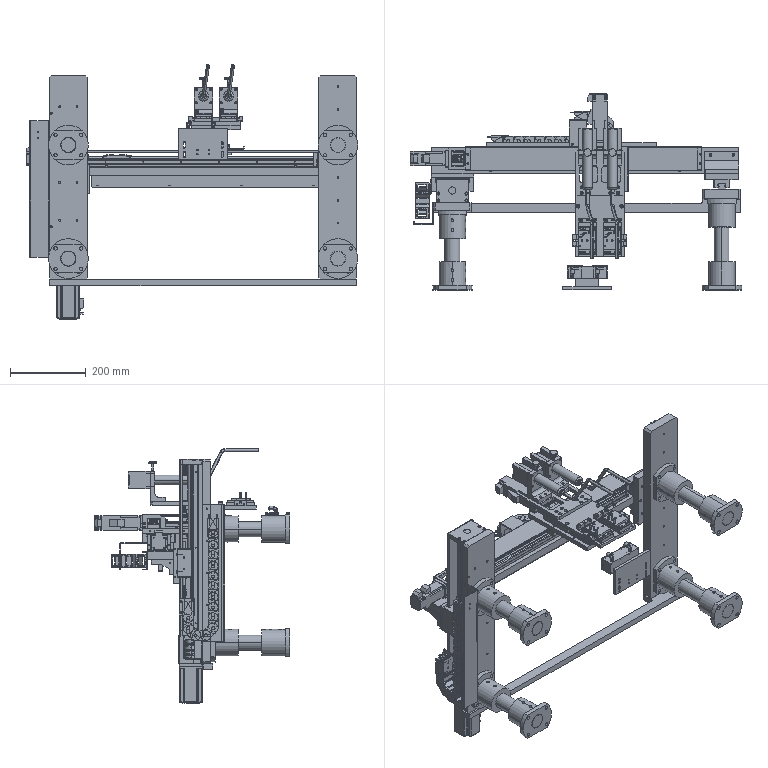Part | NX | features BREP 73 | 147 solids | 8260 faces | volume 12936713 mm3 | plane 4023 | cylinder 3422 | cone 615 | torus 130 | sphere 48 | spline 22 | commonest cylinder face diameters 8 x306 3.3 x232 4.5 x198 3 x176 5 x168 2.5 x162